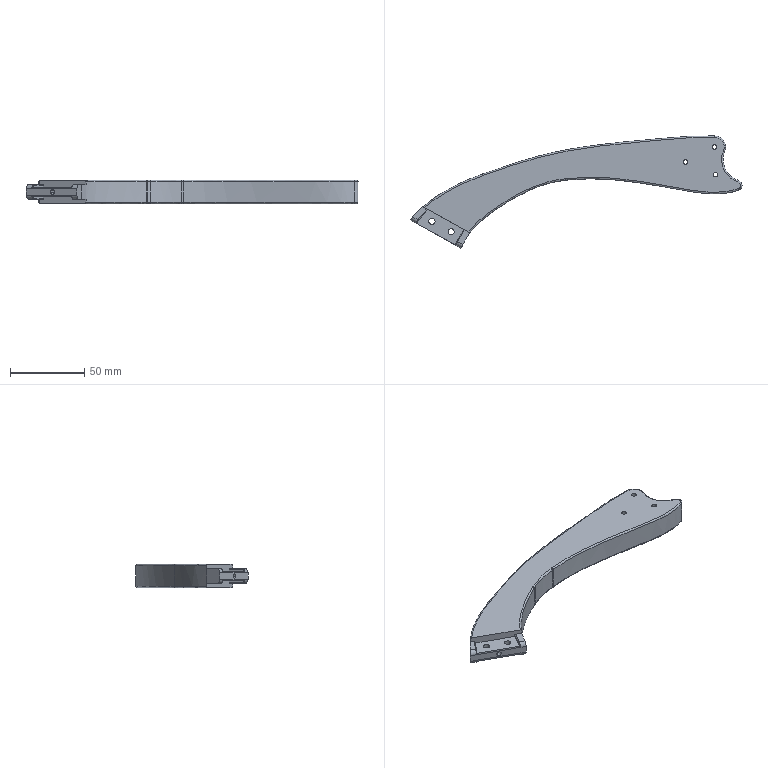Part | SolidWorks | features ICE 7, Fillet 4, Extrusion 1, MirrorPattern 1 | 1 solid | 83 faces | box 223.949 x 75.75 x 16 mm | volume 90411 mm3 | cylinder 25 | spline 23 | plane 19 | torus 16 | commonest cylinder face diameters 3.1 x6 1 x4 4.2 x4 100 x4 3 x2 5.4 x2